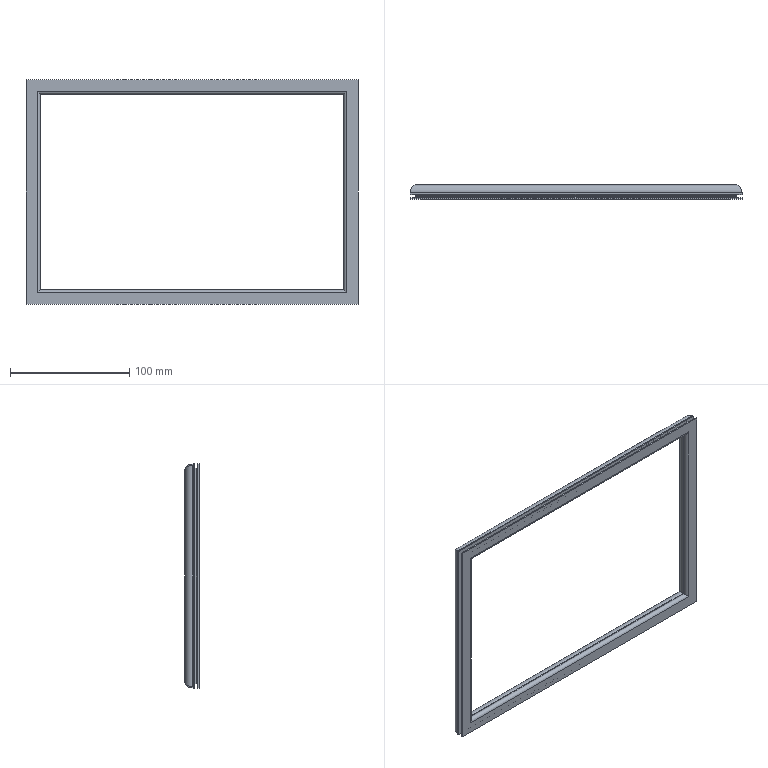Part | STEP file | _0-1000 | 1 solid | 65 faces | box 278 x 12 x 188 mm | volume 42731 mm3 | plane 49 | cylinder 16 | commonest cylinder face diameters 3 x4 5 x4 9 x4 11 x4